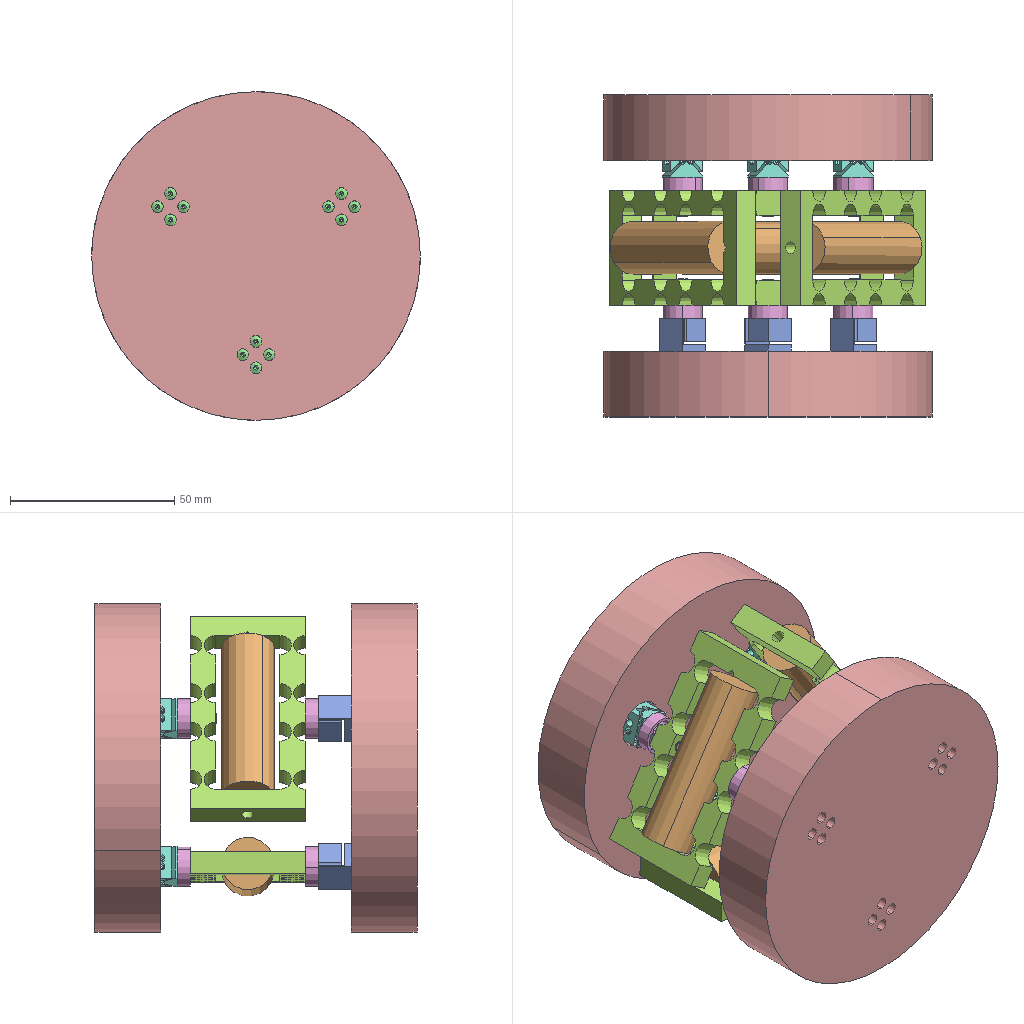Assembly | SolidWorks | 8 different items | 56 placed | box 100 x 98 x 100 mm
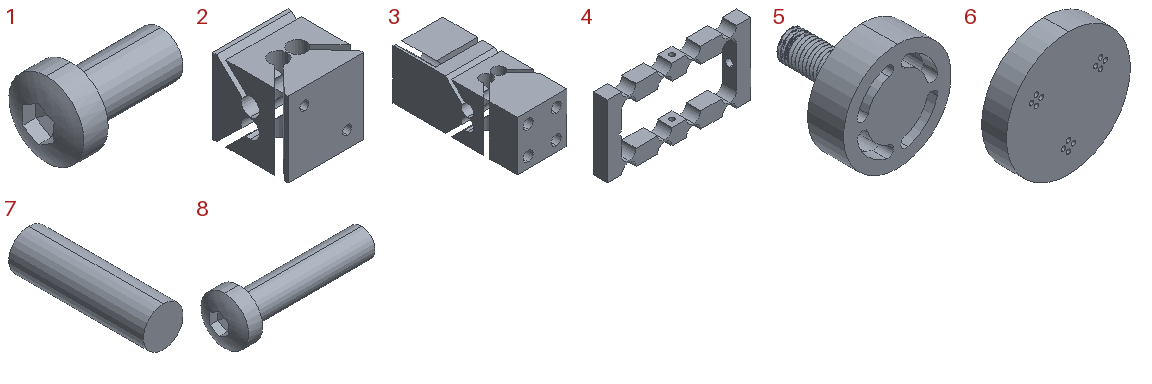Parts list (item | quantity | size | volume | features):
1 | x12 | 3.277 x 2 x 2 mm | 4.924 mm3 | features BaseBody 1, ICE 1, Scale 1
2 | x3 | 10 x 10 x 10 mm | 690.684 mm3 | features ICE 4, Extrusion 1
3 | x3 | 10 x 25 x 10 mm | 1930 mm3 | features ICE 8, Extrusion 1
4 | x3 | 70 x 7 x 35 mm | 7163 mm3 | features Extrusion 1, HoleWzd 1, ICE 1, Scale 1
5 | x6 | 12 x 12 x 12 mm | 351.083 mm3 | features ICE 3, Extrusion 1, Helix 1, Scale 1, SweepCut 1
6 | x2 | 100 x 20 x 100 mm | 148601 mm3 | features ICE 2, Cut 1, Extrusion 1
7 | x3 | 16 x 54 x 16 mm | 10857 mm3 | features Extrusion 1
8 | x24 | 10.461 x 3.5 x 3.5 mm | 39.454 mm3 | features BaseBody 1, ICE 1, MoveFace 1, Scale 1
Mates (type | each side: item.copy, entity, surface, feature):
Coincident | 6.1 face plane Cut-Extrude1 | 3.1 face plane Boss-Extrude2
Concentric | 6.1 face cylinder Cut-Extrude1 | 3.1 select_type:24
Coincident | 6.1 face plane Cut-Extrude1 | 3.2 face plane Boss-Extrude2
Concentric | 6.1 face cylinder Cut-Extrude1 | 3.2 select_type:24
Coincident | 6.1 face plane Cut-Extrude1 | 3.3 face plane Boss-Extrude2
Concentric | 6.1 face cylinder Cut-Extrude1 | 3.3 select_type:24
Concentric | 3.1 select_type:24 | 4.1 face cylinder M4 Tapped Hole1
Concentric | 3.3 select_type:24 | 4.2 face cylinder M4 Tapped Hole1
Concentric | 3.2 select_type:24 | 4.3 face cylinder M4 Tapped Hole1
Coincident | 3.2 face plane Boss-Extrude3 | 5.1 face plane Boss-Extrude1
Concentric | 3.2 select_type:24 | 5.1 face cylinder Boss-Extrude1
Coincident | 4.3 face plane Boss-Extrude1 | 5.1 face plane Boss-Extrude1
Coincident | 3.1 face plane Boss-Extrude3 | 5.2 face plane Boss-Extrude1
Concentric | 3.1 select_type:24 | 5.2 face cylinder Boss-Extrude1
Coincident | 4.1 face plane Boss-Extrude1 | 5.2 face plane Boss-Extrude1
Coincident | 3.3 face plane Boss-Extrude3 | 5.3 face plane Boss-Extrude1
Concentric | 3.3 select_type:24 | 5.3 face cylinder Boss-Extrude1
Coincident | 4.2 face plane Boss-Extrude1 | 5.3 face plane Boss-Extrude1
Concentric | 4.3 face cylinder M4 Tapped Hole1 | 5.4 face cylinder Boss-Extrude1
Coincident | 4.3 face plane Boss-Extrude1 | 5.4 face plane Boss-Extrude1
Concentric | 4.2 face cylinder M4 Tapped Hole1 | 5.5 face cylinder Boss-Extrude1
Coincident | 4.2 face plane Boss-Extrude1 | 5.5 face plane Boss-Extrude1
Concentric | 4.1 face cylinder M4 Tapped Hole1 | 5.6 face cylinder Boss-Extrude1
Coincident | 4.1 face plane Boss-Extrude1 | 5.6 face plane Boss-Extrude1
Concentric | 5.6 face cylinder Boss-Extrude1 | 2.1 select_type:24
Coincident | 5.6 face plane Boss-Extrude1 | 2.1 face plane Boss-Extrude1
Concentric | 5.4 face cylinder Boss-Extrude1 | 2.2 select_type:24
Coincident | 5.4 face plane Boss-Extrude1 | 2.2 face plane Boss-Extrude1
Concentric | 5.5 face cylinder Boss-Extrude1 | 2.3 select_type:24
Coincident | 5.5 face plane Boss-Extrude1 | 2.3 face plane Boss-Extrude1
Concentric | 6.1 face cylinder Boss-Extrude1 | 6.2 face cylinder Boss-Extrude1
Concentric | 2.2 select_type:24 | 6.2 face cylinder Cut-Extrude1
DistanceDim | 2.2 face plane Boss-Extrude1 | 6.2 face plane Cut-Extrude1
Concentric | 4.3 edge | 7.1 face cylinder Boss-Extrude1
Coincident | 4.3 face plane Boss-Extrude1 | 7.1 face plane Boss-Extrude1
Concentric | 4.1 face cylinder Cut-Extrude1 | 7.2 face cylinder Boss-Extrude1
Coincident | 4.1 face plane Boss-Extrude1 | 7.2 face plane Boss-Extrude1
Concentric | 4.2 face cylinder Cut-Extrude1 | 7.3 face cylinder Boss-Extrude1
Coincident | 4.2 face plane Boss-Extrude1 | 7.3 face plane Boss-Extrude1
Concentric | 3.1 face cylinder Cut-Extrude6 | 1.1 face cylinder Input1
Coincident | 5.2 face plane Cut-Extrude2 | 1.1 face plane Input1
Concentric | 3.1 face cylinder Cut-Extrude6 | 1.2 face cylinder Input1
Coincident | 5.2 face plane Cut-Extrude2 | 1.2 face plane Input1
Concentric | 3.2 face cylinder Cut-Extrude6 | 1.3 face cylinder Input1
Coincident | 5.1 face plane Cut-Extrude2 | 1.3 face plane Input1
Concentric | 3.2 face cylinder Cut-Extrude6 | 1.4 face cylinder Input1
Coincident | 5.1 face plane Cut-Extrude2 | 1.4 face plane Input1
Concentric | 3.3 face cylinder Cut-Extrude6 | 1.5 face cylinder Input1
Coincident | 5.3 face plane Cut-Extrude2 | 1.5 face plane Input1
Concentric | 3.3 face cylinder Cut-Extrude6 | 1.6 face cylinder Input1
Coincident | 5.3 face plane Cut-Extrude2 | 1.6 face plane Input1
Concentric | 2.2 face cylinder Cut-Extrude3 | 1.7 face cylinder Input1
Coincident | 5.4 face plane Cut-Extrude2 | 1.7 face plane Input1
Concentric | 2.2 face cylinder Cut-Extrude3 | 1.8 face cylinder Input1
Coincident | 5.4 face plane Cut-Extrude2 | 1.8 face plane Input1
Concentric | 2.3 face cylinder Cut-Extrude3 | 1.9 face cylinder Input1
Coincident | 5.5 face plane Cut-Extrude2 | 1.9 face plane Input1
Concentric | 2.3 face cylinder Cut-Extrude3 | 1.10 face cylinder Input1
Coincident | 5.5 face plane Cut-Extrude2 | 1.10 face plane Input1
Concentric | 2.1 face cylinder Cut-Extrude3 | 1.11 face cylinder Input1
Coincident | 5.6 face plane Cut-Extrude2 | 1.11 face plane Input1
Concentric | 2.1 face cylinder Cut-Extrude3 | 1.12 face cylinder Input1
Coincident | 5.6 face plane Cut-Extrude2 | 1.12 face plane Input1
Concentric | 6.1 face cylinder Cut-Extrude2 | 3.2 face cylinder Cut-Extrude5
Concentric | 6.1 face cylinder Cut-Extrude2 | 3.1 face cylinder Cut-Extrude5
Concentric | 6.1 face cylinder Cut-Extrude2 | 3.3 face cylinder Cut-Extrude5
Concentric | 2.3 face cylinder Cut-Extrude4 | 6.2 face cylinder Cut-Extrude2
Concentric | 2.1 face cylinder Cut-Extrude4 | 6.2 face cylinder Cut-Extrude2
Concentric | 6.1 face cylinder Cut-Extrude3 | 8.1 face cylinder Input1
Coincident | 6.1 face plane Cut-Extrude3 | 8.1 face plane Input1
Concentric | 6.1 face cylinder Cut-Extrude3 | 8.2 face cylinder Input1
Coincident | 6.1 face plane Cut-Extrude3 | 8.2 face plane Input1
Concentric | 6.1 face cylinder Cut-Extrude3 | 8.3 face cylinder Input1
Coincident | 6.1 face plane Cut-Extrude3 | 8.3 face plane Input1
Concentric | 6.1 face cylinder Cut-Extrude3 | 8.4 face cylinder Input1
Coincident | 6.1 face plane Cut-Extrude3 | 8.4 face plane Input1
Concentric | 6.1 face cylinder Cut-Extrude3 | 8.5 face cylinder Input1
Coincident | 6.1 face plane Cut-Extrude3 | 8.5 face plane Input1
Concentric | 6.1 face cylinder Cut-Extrude3 | 8.6 face cylinder Input1
Coincident | 6.1 face plane Cut-Extrude3 | 8.6 face plane Input1
Concentric | 6.1 face cylinder Cut-Extrude3 | 8.7 face cylinder Input1
Coincident | 6.1 face plane Cut-Extrude3 | 8.7 face plane Input1
Concentric | 6.1 face cylinder Cut-Extrude3 | 8.8 face cylinder Input1
Coincident | 6.1 face plane Cut-Extrude3 | 8.8 face plane Input1
Concentric | 6.1 face cylinder Cut-Extrude3 | 8.9 face cylinder Input1
Coincident | 6.1 face plane Cut-Extrude3 | 8.9 face plane Input1
Concentric | 6.1 face cylinder Cut-Extrude3 | 8.10 face cylinder Input1
Coincident | 6.1 face plane Cut-Extrude3 | 8.10 face plane Input1
Concentric | 6.1 face cylinder Cut-Extrude3 | 8.11 face cylinder Input1
Coincident | 6.1 face plane Cut-Extrude3 | 8.11 face plane Input1
Concentric | 6.1 face cylinder Cut-Extrude3 | 8.12 face cylinder Input1
Coincident | 6.1 face plane Cut-Extrude3 | 8.12 face plane Input1
Concentric | 6.2 face cylinder Cut-Extrude3 | 8.13 face cylinder Input1
Coincident | 6.2 face plane Cut-Extrude3 | 8.13 face plane Input1
Concentric | 6.2 face cylinder Cut-Extrude3 | 8.14 face cylinder Input1
Coincident | 6.2 face plane Cut-Extrude3 | 8.14 face plane Input1
Concentric | 6.2 face cylinder Cut-Extrude3 | 8.15 face cylinder Input1
Coincident | 6.2 face plane Cut-Extrude3 | 8.15 face plane Input1
Concentric | 6.2 face cylinder Cut-Extrude3 | 8.16 face cylinder Input1
Coincident | 6.2 face plane Cut-Extrude3 | 8.16 face plane Input1
Concentric | 6.2 face cylinder Cut-Extrude3 | 8.17 face cylinder Input1
Coincident | 6.2 face plane Cut-Extrude3 | 8.17 face plane Input1
Concentric | 6.2 face cylinder Cut-Extrude3 | 8.18 face cylinder Input1
Coincident | 6.2 face plane Cut-Extrude3 | 8.18 face plane Input1
Concentric | 6.2 face cylinder Cut-Extrude3 | 8.19 face cylinder Input1
Coincident | 6.2 face plane Cut-Extrude3 | 8.19 face plane Input1
Concentric | 6.2 face cylinder Cut-Extrude3 | 8.20 face cylinder Input1
Coincident | 6.2 face plane Cut-Extrude3 | 8.20 face plane Input1
Concentric | 6.2 face cylinder Cut-Extrude3 | 8.21 face cylinder Input1
Coincident | 6.2 face plane Cut-Extrude3 | 8.21 face plane Input1
Concentric | 6.2 face cylinder Cut-Extrude3 | 8.22 face cylinder Input1
Coincident | 6.2 face plane Cut-Extrude3 | 8.22 face plane Input1
Concentric | 6.2 face cylinder Cut-Extrude3 | 8.23 face cylinder Input1
Coincident | 6.2 face plane Cut-Extrude3 | 8.23 face plane Input1
Concentric | 6.2 face cylinder Cut-Extrude3 | 8.24 face cylinder Input1
Coincident | 6.2 face plane Cut-Extrude3 | 8.24 face plane Input1